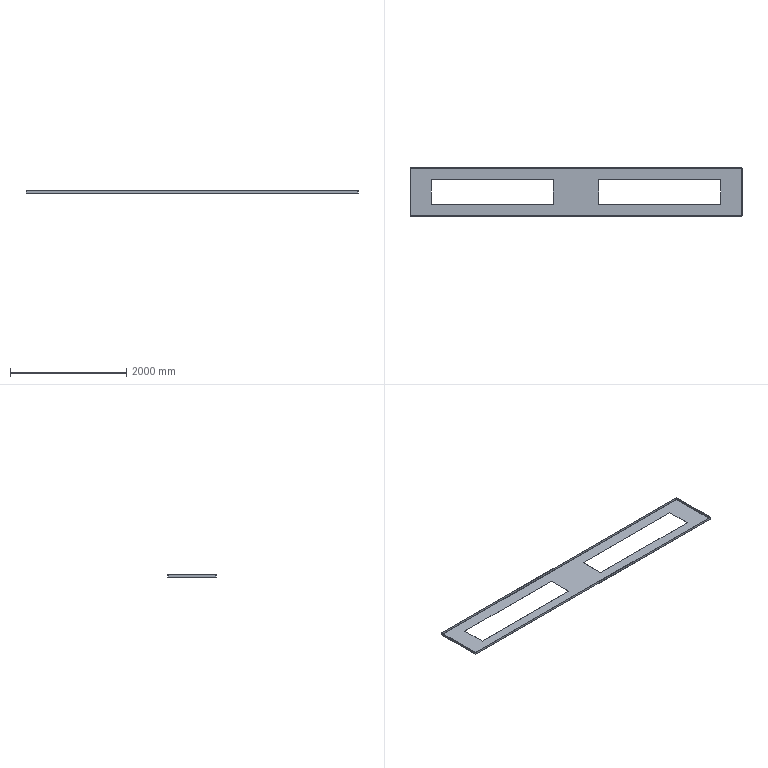Part | SolidWorks | features Cut 1, EdgeFlange 1, FlatPattern 1, SMBaseFlange 1, SheetMetal 1 | 1 solid | 46 faces | box 5700 x 825 x 40 mm | volume 6847674 mm3 | plane 30 | spline 8 | cylinder 8 | commonest cylinder face diameters 1.473 x4 5.473 x4